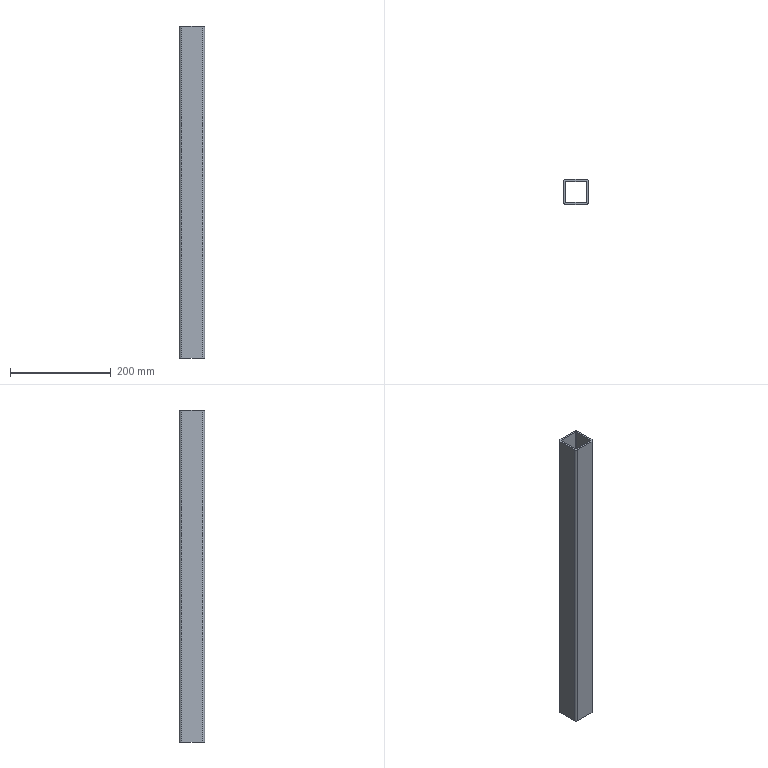Part | STEP file | 冲床-300配套压波_id966_x_t | 1 solid | 18 faces | box 50 x 50 x 660 mm | volume 472163 mm3 | plane 10 | cylinder 8 | commonest cylinder face diameters 2 x4 10 x4
STEP:
#1=CARTESIAN_POINT('',(1519.,-235.,-70.));
#2=VERTEX_POINT('',#1);
#3=CARTESIAN_POINT('',(1519.,-275.,-70.));
#4=VERTEX_POINT('',#3);
#5=CARTESIAN_POINT('',(1519.,-30.,-70.));
#6=DIRECTION('',(0.,-1.,0.));
#7=VECTOR('',#6,1.);
#8=LINE('',#5,#7);
#9=EDGE_CURVE('',#2,#4,#8,.T.);
#10=ORIENTED_EDGE('',*,*,#9,.F.);
#11=CARTESIAN_POINT('',(1520.,-234.,-70.));
#12=VERTEX_POINT('',#11);
#13=CARTESIAN_POINT('',(1520.,-235.,-70.));
#14=DIRECTION('',(0.,0.,1.));
#15=DIRECTION('',(1.,0.,0.));
#16=AXIS2_PLACEMENT_3D('',#13,#14,#15);
#17=CIRCLE('',#16,1.);
#18=EDGE_CURVE('',#12,#2,#17,.T.);
#19=ORIENTED_EDGE('',*,*,#18,.F.);
#20=CARTESIAN_POINT('',(1560.,-234.,-70.));
#21=VERTEX_POINT('',#20);
#22=CARTESIAN_POINT('',(365.,-234.,-70.));
#23=DIRECTION('',(-1.,0.,0.));
#24=VECTOR('',#23,1.);
#25=LINE('',#22,#24);
#26=EDGE_CURVE('',#21,#12,#25,.T.);
#27=ORIENTED_EDGE('',*,*,#26,.F.);
#28=CARTESIAN_POINT('',(1561.,-235.,-70.));
#29=VERTEX_POINT('',#28);
#30=CARTESIAN_POINT('',(1560.,-235.,-70.));
#31=DIRECTION('',(0.,0.,1.));
#32=DIRECTION('',(1.,0.,0.));
#33=AXIS2_PLACEMENT_3D('',#30,#31,#32);
#34=CIRCLE('',#33,1.);
#35=EDGE_CURVE('',#29,#21,#34,.T.);
#36=ORIENTED_EDGE('',*,*,#35,.F.);
#37=CARTESIAN_POINT('',(1561.,-275.,-70.));
#38=VERTEX_POINT('',#37);
#39=CARTESIAN_POINT('',(1561.,-30.,-70.));
#40=DIRECTION('',(0.,1.,0.));
#41=VECTOR('',#40,1.);
#42=LINE('',#39,#41);
#43=EDGE_CURVE('',#38,#29,#42,.T.);
#44=ORIENTED_EDGE('',*,*,#43,.F.);
#45=CARTESIAN_POINT('',(1560.,-276.,-70.));
#46=VERTEX_POINT('',#45);
#47=CARTESIAN_POINT('',(1560.,-275.,-70.));
#48=DIRECTION('',(0.,0.,1.));
#49=DIRECTION('',(1.,0.,0.));
#50=AXIS2_PLACEMENT_3D('',#47,#48,#49);
#51=CIRCLE('',#50,1.);
#52=EDGE_CURVE('',#46,#38,#51,.T.);
#53=ORIENTED_EDGE('',*,*,#52,.F.);
#54=CARTESIAN_POINT('',(1520.,-276.,-70.));
#55=VERTEX_POINT('',#54);
#56=CARTESIAN_POINT('',(365.,-276.,-70.));
#57=DIRECTION('',(1.,0.,0.));
#58=VECTOR('',#57,1.);
#59=LINE('',#56,#58);
#60=EDGE_CURVE('',#55,#46,#59,.T.);
#61=ORIENTED_EDGE('',*,*,#60,.F.);
#62=CARTESIAN_POINT('',(1520.,-275.,-70.));
#63=DIRECTION('',(0.,0.,1.));
#64=DIRECTION('',(1.,0.,0.));
#65=AXIS2_PLACEMENT_3D('',#62,#63,#64);
#66=CIRCLE('',#65,1.);
#67=EDGE_CURVE('',#4,#55,#66,.T.);
#68=ORIENTED_EDGE('',*,*,#67,.F.);
#69=EDGE_LOOP('',(#10,#19,#27,#36,#44,#53,#61,#68));
#70=FACE_BOUND('',#69,.T.);
#71=CARTESIAN_POINT('',(1515.,-235.,-70.));
#72=VERTEX_POINT('',#71);
#73=CARTESIAN_POINT('',(1515.,-275.,-70.));
#74=VERTEX_POINT('',#73);
#75=CARTESIAN_POINT('',(1515.,-30.,-70.));
#76=DIRECTION('',(0.,-1.,0.));
#77=VECTOR('',#76,1.);
#78=LINE('',#75,#77);
#79=EDGE_CURVE('',#72,#74,#78,.T.);
#80=ORIENTED_EDGE('',*,*,#79,.T.);
#81=CARTESIAN_POINT('',(1520.,-280.,-70.));
#82=VERTEX_POINT('',#81);
#83=CARTESIAN_POINT('',(1520.,-275.,-70.));
#84=DIRECTION('',(0.,0.,1.));
#85=DIRECTION('',(1.,0.,0.));
#86=AXIS2_PLACEMENT_3D('',#83,#84,#85);
#87=CIRCLE('',#86,5.);
#88=EDGE_CURVE('',#74,#82,#87,.T.);
#89=ORIENTED_EDGE('',*,*,#88,.T.);
#90=CARTESIAN_POINT('',(1560.,-280.,-70.));
#91=VERTEX_POINT('',#90);
#92=CARTESIAN_POINT('',(365.,-280.,-70.));
#93=DIRECTION('',(1.,0.,0.));
#94=VECTOR('',#93,1.);
#95=LINE('',#92,#94);
#96=EDGE_CURVE('',#82,#91,#95,.T.);
#97=ORIENTED_EDGE('',*,*,#96,.T.);
#98=CARTESIAN_POINT('',(1565.,-275.,-70.));
#99=VERTEX_POINT('',#98);
#100=CARTESIAN_POINT('',(1560.,-275.,-70.));
#101=DIRECTION('',(0.,0.,1.));
#102=DIRECTION('',(1.,0.,0.));
#103=AXIS2_PLACEMENT_3D('',#100,#101,#102);
#104=CIRCLE('',#103,5.);
#105=EDGE_CURVE('',#91,#99,#104,.T.);
#106=ORIENTED_EDGE('',*,*,#105,.T.);
#107=CARTESIAN_POINT('',(1565.,-235.,-70.));
#108=VERTEX_POINT('',#107);
#109=CARTESIAN_POINT('',(1565.,-30.,-70.));
#110=DIRECTION('',(0.,1.,0.));
#111=VECTOR('',#110,1.);
#112=LINE('',#109,#111);
#113=EDGE_CURVE('',#99,#108,#112,.T.);
#114=ORIENTED_EDGE('',*,*,#113,.T.);
#115=CARTESIAN_POINT('',(1560.,-230.,-70.));
#116=VERTEX_POINT('',#115);
#117=CARTESIAN_POINT('',(1560.,-235.,-70.));
#118=DIRECTION('',(0.,0.,1.));
#119=DIRECTION('',(1.,0.,0.));
#120=AXIS2_PLACEMENT_3D('',#117,#118,#119);
#121=CIRCLE('',#120,5.);
#122=EDGE_CURVE('',#108,#116,#121,.T.);
#123=ORIENTED_EDGE('',*,*,#122,.T.);
#124=CARTESIAN_POINT('',(1520.,-230.,-70.));
#125=VERTEX_POINT('',#124);
#126=CARTESIAN_POINT('',(365.,-230.,-70.));
#127=DIRECTION('',(-1.,0.,0.));
#128=VECTOR('',#127,1.);
#129=LINE('',#126,#128);
#130=EDGE_CURVE('',#116,#125,#129,.T.);
#131=ORIENTED_EDGE('',*,*,#130,.T.);
#132=CARTESIAN_POINT('',(1520.,-235.,-70.));
#133=DIRECTION('',(0.,0.,1.));
#134=DIRECTION('',(1.,0.,0.));
#135=AXIS2_PLACEMENT_3D('',#132,#133,#134);
#136=CIRCLE('',#135,5.);
#137=EDGE_CURVE('',#125,#72,#136,.T.);
#138=ORIENTED_EDGE('',*,*,#137,.T.);
#139=EDGE_LOOP('',(#80,#89,#97,#106,#114,#123,#131,#138));
#140=FACE_BOUND('',#139,.T.);
#141=CARTESIAN_POINT('',(365.,-30.,-70.));
#142=DIRECTION('',(0.,0.,1.));
#143=DIRECTION('',(1.,0.,0.));
#144=AXIS2_PLACEMENT_3D('',#141,#142,#143);
#145=PLANE('',#144);
#146=ADVANCED_FACE('',(#70,#140),#145,.T.);
#147=CARTESIAN_POINT('',(1520.,-230.,-730.));
#148=VERTEX_POINT('',#147);
#149=CARTESIAN_POINT('',(1520.,-230.,-740.));
#150=DIRECTION('',(0.,0.,-1.));
#151=VECTOR('',#150,1.);
#152=LINE('',#149,#151);
#153=EDGE_CURVE('',#125,#148,#152,.T.);
#154=ORIENTED_EDGE('',*,*,#153,.T.);
#155=CARTESIAN_POINT('',(1515.,-235.,-730.));
#156=VERTEX_POINT('',#155);
#157=CARTESIAN_POINT('',(1520.,-235.,-730.));
#158=DIRECTION('',(0.,0.,1.));
#159=DIRECTION('',(1.,0.,0.));
#160=AXIS2_PLACEMENT_3D('',#157,#158,#159);
#161=CIRCLE('',#160,5.);
#162=EDGE_CURVE('',#148,#156,#161,.T.);
#163=ORIENTED_EDGE('',*,*,#162,.T.);
#164=CARTESIAN_POINT('',(1515.,-235.,-740.));
#165=DIRECTION('',(0.,0.,-1.));
#166=VECTOR('',#165,1.);
#167=LINE('',#164,#166);
#168=EDGE_CURVE('',#72,#156,#167,.T.);
#169=ORIENTED_EDGE('',*,*,#168,.F.);
#170=ORIENTED_EDGE('',*,*,#137,.F.);
#171=EDGE_LOOP('',(#154,#163,#169,#170));
#172=FACE_OUTER_BOUND('',#171,.T.);
#173=CARTESIAN_POINT('',(1520.,-235.,-740.));
#174=DIRECTION('',(0.,0.,1.));
#175=DIRECTION('',(1.,0.,0.));
#176=AXIS2_PLACEMENT_3D('',#173,#174,#175);
#177=CYLINDRICAL_SURFACE('',#176,5.);
#178=ADVANCED_FACE('',(#172),#177,.T.);
#179=CARTESIAN_POINT('',(1560.,-230.,-730.));
#180=VERTEX_POINT('',#179);
#181=CARTESIAN_POINT('',(1560.,-230.,-740.));
#182=DIRECTION('',(0.,0.,-1.));
#183=VECTOR('',#182,1.);
#184=LINE('',#181,#183);
#185=EDGE_CURVE('',#116,#180,#184,.T.);
#186=ORIENTED_EDGE('',*,*,#185,.T.);
#187=CARTESIAN_POINT('',(1520.,-230.,-730.));
#188=DIRECTION('',(-1.,0.,0.));
#189=VECTOR('',#188,1.);
#190=LINE('',#187,#189);
#191=EDGE_CURVE('',#180,#148,#190,.T.);
#192=ORIENTED_EDGE('',*,*,#191,.T.);
#193=ORIENTED_EDGE('',*,*,#153,.F.);
#194=ORIENTED_EDGE('',*,*,#130,.F.);
#195=EDGE_LOOP('',(#186,#192,#193,#194));
#196=FACE_OUTER_BOUND('',#195,.T.);
#197=CARTESIAN_POINT('',(1520.,-230.,-740.));
#198=DIRECTION('',(0.,1.,0.));
#199=DIRECTION('',(1.,0.,0.));
#200=AXIS2_PLACEMENT_3D('',#197,#198,#199);
#201=PLANE('',#200);
#202=ADVANCED_FACE('',(#196),#201,.T.);
#203=CARTESIAN_POINT('',(1565.,-235.,-730.));
#204=VERTEX_POINT('',#203);
#205=CARTESIAN_POINT('',(1565.,-235.,-740.));
#206=DIRECTION('',(0.,0.,-1.));
#207=VECTOR('',#206,1.);
#208=LINE('',#205,#207);
#209=EDGE_CURVE('',#108,#204,#208,.T.);
#210=ORIENTED_EDGE('',*,*,#209,.T.);
#211=CARTESIAN_POINT('',(1560.,-235.,-730.));
#212=DIRECTION('',(0.,0.,1.));
#213=DIRECTION('',(1.,0.,0.));
#214=AXIS2_PLACEMENT_3D('',#211,#212,#213);
#215=CIRCLE('',#214,5.);
#216=EDGE_CURVE('',#204,#180,#215,.T.);
#217=ORIENTED_EDGE('',*,*,#216,.T.);
#218=ORIENTED_EDGE('',*,*,#185,.F.);
#219=ORIENTED_EDGE('',*,*,#122,.F.);
#220=EDGE_LOOP('',(#210,#217,#218,#219));
#221=FACE_OUTER_BOUND('',#220,.T.);
#222=CARTESIAN_POINT('',(1560.,-235.,-740.));
#223=DIRECTION('',(0.,0.,1.));
#224=DIRECTION('',(1.,0.,0.));
#225=AXIS2_PLACEMENT_3D('',#222,#223,#224);
#226=CYLINDRICAL_SURFACE('',#225,5.);
#227=ADVANCED_FACE('',(#221),#226,.T.);
#228=CARTESIAN_POINT('',(1565.,-275.,-730.));
#229=VERTEX_POINT('',#228);
#230=CARTESIAN_POINT('',(1565.,-275.,-740.));
#231=DIRECTION('',(0.,0.,-1.));
#232=VECTOR('',#231,1.);
#233=LINE('',#230,#232);
#234=EDGE_CURVE('',#99,#229,#233,.T.);
#235=ORIENTED_EDGE('',*,*,#234,.T.);
#236=CARTESIAN_POINT('',(1565.,-235.,-730.));
#237=DIRECTION('',(0.,1.,0.));
#238=VECTOR('',#237,1.);
#239=LINE('',#236,#238);
#240=EDGE_CURVE('',#229,#204,#239,.T.);
#241=ORIENTED_EDGE('',*,*,#240,.T.);
#242=ORIENTED_EDGE('',*,*,#209,.F.);
#243=ORIENTED_EDGE('',*,*,#113,.F.);
#244=EDGE_LOOP('',(#235,#241,#242,#243));
#245=FACE_OUTER_BOUND('',#244,.T.);
#246=CARTESIAN_POINT('',(1565.,-235.,-740.));
#247=DIRECTION('',(1.,0.,0.));
#248=DIRECTION('',(0.,0.,-1.));
#249=AXIS2_PLACEMENT_3D('',#246,#247,#248);
#250=PLANE('',#249);
#251=ADVANCED_FACE('',(#245),#250,.T.);
#252=CARTESIAN_POINT('',(1560.,-280.,-730.));
#253=VERTEX_POINT('',#252);
#254=CARTESIAN_POINT('',(1560.,-280.,-740.));
#255=DIRECTION('',(0.,0.,-1.));
#256=VECTOR('',#255,1.);
#257=LINE('',#254,#256);
#258=EDGE_CURVE('',#91,#253,#257,.T.);
#259=ORIENTED_EDGE('',*,*,#258,.T.);
#260=CARTESIAN_POINT('',(1560.,-275.,-730.));
#261=DIRECTION('',(0.,0.,1.));
#262=DIRECTION('',(1.,0.,0.));
#263=AXIS2_PLACEMENT_3D('',#260,#261,#262);
#264=CIRCLE('',#263,5.);
#265=EDGE_CURVE('',#253,#229,#264,.T.);
#266=ORIENTED_EDGE('',*,*,#265,.T.);
#267=ORIENTED_EDGE('',*,*,#234,.F.);
#268=ORIENTED_EDGE('',*,*,#105,.F.);
#269=EDGE_LOOP('',(#259,#266,#267,#268));
#270=FACE_OUTER_BOUND('',#269,.T.);
#271=CARTESIAN_POINT('',(1560.,-275.,-740.));
#272=DIRECTION('',(0.,0.,1.));
#273=DIRECTION('',(1.,0.,0.));
#274=AXIS2_PLACEMENT_3D('',#271,#272,#273);
#275=CYLINDRICAL_SURFACE('',#274,5.);
#276=ADVANCED_FACE('',(#270),#275,.T.);
#277=CARTESIAN_POINT('',(1519.,-275.,-730.));
#278=VERTEX_POINT('',#277);
#279=CARTESIAN_POINT('',(1520.,-276.,-730.));
#280=VERTEX_POINT('',#279);
#281=CARTESIAN_POINT('',(1520.,-275.,-730.));
#282=DIRECTION('',(0.,0.,1.));
#283=DIRECTION('',(1.,0.,0.));
#284=AXIS2_PLACEMENT_3D('',#281,#282,#283);
#285=CIRCLE('',#284,1.);
#286=EDGE_CURVE('',#278,#280,#285,.T.);
#287=ORIENTED_EDGE('',*,*,#286,.T.);
#288=CARTESIAN_POINT('',(1560.,-276.,-730.));
#289=VERTEX_POINT('',#288);
#290=CARTESIAN_POINT('',(1520.,-276.,-730.));
#291=DIRECTION('',(1.,0.,0.));
#292=VECTOR('',#291,1.);
#293=LINE('',#290,#292);
#294=EDGE_CURVE('',#280,#289,#293,.T.);
#295=ORIENTED_EDGE('',*,*,#294,.T.);
#296=CARTESIAN_POINT('',(1561.,-275.,-730.));
#297=VERTEX_POINT('',#296);
#298=CARTESIAN_POINT('',(1560.,-275.,-730.));
#299=DIRECTION('',(0.,0.,1.));
#300=DIRECTION('',(1.,0.,0.));
#301=AXIS2_PLACEMENT_3D('',#298,#299,#300);
#302=CIRCLE('',#301,1.);
#303=EDGE_CURVE('',#289,#297,#302,.T.);
#304=ORIENTED_EDGE('',*,*,#303,.T.);
#305=CARTESIAN_POINT('',(1561.,-235.,-730.));
#306=VERTEX_POINT('',#305);
#307=CARTESIAN_POINT('',(1561.,-235.,-730.));
#308=DIRECTION('',(0.,1.,0.));
#309=VECTOR('',#308,1.);
#310=LINE('',#307,#309);
#311=EDGE_CURVE('',#297,#306,#310,.T.);
#312=ORIENTED_EDGE('',*,*,#311,.T.);
#313=CARTESIAN_POINT('',(1560.,-234.,-730.));
#314=VERTEX_POINT('',#313);
#315=CARTESIAN_POINT('',(1560.,-235.,-730.));
#316=DIRECTION('',(0.,0.,1.));
#317=DIRECTION('',(1.,0.,0.));
#318=AXIS2_PLACEMENT_3D('',#315,#316,#317);
#319=CIRCLE('',#318,1.);
#320=EDGE_CURVE('',#306,#314,#319,.T.);
#321=ORIENTED_EDGE('',*,*,#320,.T.);
#322=CARTESIAN_POINT('',(1520.,-234.,-730.));
#323=VERTEX_POINT('',#322);
#324=CARTESIAN_POINT('',(1520.,-234.,-730.));
#325=DIRECTION('',(-1.,0.,0.));
#326=VECTOR('',#325,1.);
#327=LINE('',#324,#326);
#328=EDGE_CURVE('',#314,#323,#327,.T.);
#329=ORIENTED_EDGE('',*,*,#328,.T.);
#330=CARTESIAN_POINT('',(1519.,-235.,-730.));
#331=VERTEX_POINT('',#330);
#332=CARTESIAN_POINT('',(1520.,-235.,-730.));
#333=DIRECTION('',(0.,0.,1.));
#334=DIRECTION('',(1.,0.,0.));
#335=AXIS2_PLACEMENT_3D('',#332,#333,#334);
#336=CIRCLE('',#335,1.);
#337=EDGE_CURVE('',#323,#331,#336,.T.);
#338=ORIENTED_EDGE('',*,*,#337,.T.);
#339=CARTESIAN_POINT('',(1519.,-235.,-730.));
#340=DIRECTION('',(0.,-1.,0.));
#341=VECTOR('',#340,1.);
#342=LINE('',#339,#341);
#343=EDGE_CURVE('',#331,#278,#342,.T.);
#344=ORIENTED_EDGE('',*,*,#343,.T.);
#345=EDGE_LOOP('',(#287,#295,#304,#312,#321,#329,#338,#344));
#346=FACE_BOUND('',#345,.T.);
#347=CARTESIAN_POINT('',(1515.,-275.,-730.));
#348=VERTEX_POINT('',#347);
#349=CARTESIAN_POINT('',(1515.,-235.,-730.));
#350=DIRECTION('',(0.,-1.,0.));
#351=VECTOR('',#350,1.);
#352=LINE('',#349,#351);
#353=EDGE_CURVE('',#156,#348,#352,.T.);
#354=ORIENTED_EDGE('',*,*,#353,.F.);
#355=ORIENTED_EDGE('',*,*,#162,.F.);
#356=ORIENTED_EDGE('',*,*,#191,.F.);
#357=ORIENTED_EDGE('',*,*,#216,.F.);
#358=ORIENTED_EDGE('',*,*,#240,.F.);
#359=ORIENTED_EDGE('',*,*,#265,.F.);
#360=CARTESIAN_POINT('',(1520.,-280.,-730.));
#361=VERTEX_POINT('',#360);
#362=CARTESIAN_POINT('',(1520.,-280.,-730.));
#363=DIRECTION('',(1.,0.,0.));
#364=VECTOR('',#363,1.);
#365=LINE('',#362,#364);
#366=EDGE_CURVE('',#361,#253,#365,.T.);
#367=ORIENTED_EDGE('',*,*,#366,.F.);
#368=CARTESIAN_POINT('',(1520.,-275.,-730.));
#369=DIRECTION('',(0.,0.,1.));
#370=DIRECTION('',(1.,0.,0.));
#371=AXIS2_PLACEMENT_3D('',#368,#369,#370);
#372=CIRCLE('',#371,5.);
#373=EDGE_CURVE('',#348,#361,#372,.T.);
#374=ORIENTED_EDGE('',*,*,#373,.F.);
#375=EDGE_LOOP('',(#354,#355,#356,#357,#358,#359,#367,#374));
#376=FACE_BOUND('',#375,.T.);
#377=CARTESIAN_POINT('',(1520.,-235.,-730.));
#378=DIRECTION('',(0.,0.,1.));
#379=DIRECTION('',(1.,0.,0.));
#380=AXIS2_PLACEMENT_3D('',#377,#378,#379);
#381=PLANE('',#380);
#382=ADVANCED_FACE('',(#346,#376),#381,.F.);
#383=CARTESIAN_POINT('',(1520.,-280.,-740.));
#384=DIRECTION('',(0.,0.,-1.));
#385=VECTOR('',#384,1.);
#386=LINE('',#383,#385);
#387=EDGE_CURVE('',#82,#361,#386,.T.);
#388=ORIENTED_EDGE('',*,*,#387,.T.);
#389=ORIENTED_EDGE('',*,*,#366,.T.);
#390=ORIENTED_EDGE('',*,*,#258,.F.);
#391=ORIENTED_EDGE('',*,*,#96,.F.);
#392=EDGE_LOOP('',(#388,#389,#390,#391));
#393=FACE_OUTER_BOUND('',#392,.T.);
#394=CARTESIAN_POINT('',(1560.,-280.,-740.));
#395=DIRECTION('',(0.,-1.,0.));
#396=DIRECTION('',(-1.,0.,0.));
#397=AXIS2_PLACEMENT_3D('',#394,#395,#396);
#398=PLANE('',#397);
#399=ADVANCED_FACE('',(#393),#398,.T.);
#400=ORIENTED_EDGE('',*,*,#168,.T.);
#401=ORIENTED_EDGE('',*,*,#353,.T.);
#402=CARTESIAN_POINT('',(1515.,-275.,-740.));
#403=DIRECTION('',(0.,0.,-1.));
#404=VECTOR('',#403,1.);
#405=LINE('',#402,#404);
#406=EDGE_CURVE('',#74,#348,#405,.T.);
#407=ORIENTED_EDGE('',*,*,#406,.F.);
#408=ORIENTED_EDGE('',*,*,#79,.F.);
#409=EDGE_LOOP('',(#400,#401,#407,#408));
#410=FACE_OUTER_BOUND('',#409,.T.);
#411=CARTESIAN_POINT('',(1515.,-275.,-740.));
#412=DIRECTION('',(-1.,0.,0.));
#413=DIRECTION('',(0.,0.,1.));
#414=AXIS2_PLACEMENT_3D('',#411,#412,#413);
#415=PLANE('',#414);
#416=ADVANCED_FACE('',(#410),#415,.T.);
#417=ORIENTED_EDGE('',*,*,#406,.T.);
#418=ORIENTED_EDGE('',*,*,#373,.T.);
#419=ORIENTED_EDGE('',*,*,#387,.F.);
#420=ORIENTED_EDGE('',*,*,#88,.F.);
#421=EDGE_LOOP('',(#417,#418,#419,#420));
#422=FACE_OUTER_BOUND('',#421,.T.);
#423=CARTESIAN_POINT('',(1520.,-275.,-740.));
#424=DIRECTION('',(0.,0.,1.));
#425=DIRECTION('',(1.,0.,0.));
#426=AXIS2_PLACEMENT_3D('',#423,#424,#425);
#427=CYLINDRICAL_SURFACE('',#426,5.);
#428=ADVANCED_FACE('',(#422),#427,.T.);
#429=CARTESIAN_POINT('',(1520.,-234.,-740.));
#430=DIRECTION('',(0.,0.,-1.));
#431=VECTOR('',#430,1.);
#432=LINE('',#429,#431);
#433=EDGE_CURVE('',#12,#323,#432,.T.);
#434=ORIENTED_EDGE('',*,*,#433,.F.);
#435=ORIENTED_EDGE('',*,*,#18,.T.);
#436=CARTESIAN_POINT('',(1519.,-235.,-740.));
#437=DIRECTION('',(0.,0.,-1.));
#438=VECTOR('',#437,1.);
#439=LINE('',#436,#438);
#440=EDGE_CURVE('',#2,#331,#439,.T.);
#441=ORIENTED_EDGE('',*,*,#440,.T.);
#442=ORIENTED_EDGE('',*,*,#337,.F.);
#443=EDGE_LOOP('',(#434,#435,#441,#442));
#444=FACE_OUTER_BOUND('',#443,.T.);
#445=CARTESIAN_POINT('',(1520.,-235.,-740.));
#446=DIRECTION('',(0.,0.,1.));
#447=DIRECTION('',(1.,0.,0.));
#448=AXIS2_PLACEMENT_3D('',#445,#446,#447);
#449=CYLINDRICAL_SURFACE('',#448,1.);
#450=ADVANCED_FACE('',(#444),#449,.F.);
#451=CARTESIAN_POINT('',(1560.,-234.,-740.));
#452=DIRECTION('',(0.,0.,-1.));
#453=VECTOR('',#452,1.);
#454=LINE('',#451,#453);
#455=EDGE_CURVE('',#21,#314,#454,.T.);
#456=ORIENTED_EDGE('',*,*,#455,.F.);
#457=ORIENTED_EDGE('',*,*,#26,.T.);
#458=ORIENTED_EDGE('',*,*,#433,.T.);
#459=ORIENTED_EDGE('',*,*,#328,.F.);
#460=EDGE_LOOP('',(#456,#457,#458,#459));
#461=FACE_OUTER_BOUND('',#460,.T.);
#462=CARTESIAN_POINT('',(1520.,-234.,-740.));
#463=DIRECTION('',(0.,1.,0.));
#464=DIRECTION('',(1.,0.,0.));
#465=AXIS2_PLACEMENT_3D('',#462,#463,#464);
#466=PLANE('',#465);
#467=ADVANCED_FACE('',(#461),#466,.F.);
#468=CARTESIAN_POINT('',(1561.,-235.,-740.));
#469=DIRECTION('',(0.,0.,-1.));
#470=VECTOR('',#469,1.);
#471=LINE('',#468,#470);
#472=EDGE_CURVE('',#29,#306,#471,.T.);
#473=ORIENTED_EDGE('',*,*,#472,.F.);
#474=ORIENTED_EDGE('',*,*,#35,.T.);
#475=ORIENTED_EDGE('',*,*,#455,.T.);
#476=ORIENTED_EDGE('',*,*,#320,.F.);
#477=EDGE_LOOP('',(#473,#474,#475,#476));
#478=FACE_OUTER_BOUND('',#477,.T.);
#479=CARTESIAN_POINT('',(1560.,-235.,-740.));
#480=DIRECTION('',(0.,0.,1.));
#481=DIRECTION('',(1.,0.,0.));
#482=AXIS2_PLACEMENT_3D('',#479,#480,#481);
#483=CYLINDRICAL_SURFACE('',#482,1.);
#484=ADVANCED_FACE('',(#478),#483,.F.);
#485=CARTESIAN_POINT('',(1561.,-275.,-740.));
#486=DIRECTION('',(0.,0.,-1.));
#487=VECTOR('',#486,1.);
#488=LINE('',#485,#487);
#489=EDGE_CURVE('',#38,#297,#488,.T.);
#490=ORIENTED_EDGE('',*,*,#489,.F.);
#491=ORIENTED_EDGE('',*,*,#43,.T.);
#492=ORIENTED_EDGE('',*,*,#472,.T.);
#493=ORIENTED_EDGE('',*,*,#311,.F.);
#494=EDGE_LOOP('',(#490,#491,#492,#493));
#495=FACE_OUTER_BOUND('',#494,.T.);
#496=CARTESIAN_POINT('',(1561.,-235.,-740.));
#497=DIRECTION('',(1.,0.,0.));
#498=DIRECTION('',(0.,0.,-1.));
#499=AXIS2_PLACEMENT_3D('',#496,#497,#498);
#500=PLANE('',#499);
#501=ADVANCED_FACE('',(#495),#500,.F.);
#502=CARTESIAN_POINT('',(1560.,-276.,-740.));
#503=DIRECTION('',(0.,0.,-1.));
#504=VECTOR('',#503,1.);
#505=LINE('',#502,#504);
#506=EDGE_CURVE('',#46,#289,#505,.T.);
#507=ORIENTED_EDGE('',*,*,#506,.F.);
#508=ORIENTED_EDGE('',*,*,#52,.T.);
#509=ORIENTED_EDGE('',*,*,#489,.T.);
#510=ORIENTED_EDGE('',*,*,#303,.F.);
#511=EDGE_LOOP('',(#507,#508,#509,#510));
#512=FACE_OUTER_BOUND('',#511,.T.);
#513=CARTESIAN_POINT('',(1560.,-275.,-740.));
#514=DIRECTION('',(0.,0.,1.));
#515=DIRECTION('',(1.,0.,0.));
#516=AXIS2_PLACEMENT_3D('',#513,#514,#515);
#517=CYLINDRICAL_SURFACE('',#516,1.);
#518=ADVANCED_FACE('',(#512),#517,.F.);
#519=CARTESIAN_POINT('',(1520.,-276.,-740.));
#520=DIRECTION('',(0.,0.,-1.));
#521=VECTOR('',#520,1.);
#522=LINE('',#519,#521);
#523=EDGE_CURVE('',#55,#280,#522,.T.);
#524=ORIENTED_EDGE('',*,*,#523,.F.);
#525=ORIENTED_EDGE('',*,*,#60,.T.);
#526=ORIENTED_EDGE('',*,*,#506,.T.);
#527=ORIENTED_EDGE('',*,*,#294,.F.);
#528=EDGE_LOOP('',(#524,#525,#526,#527));
#529=FACE_OUTER_BOUND('',#528,.T.);
#530=CARTESIAN_POINT('',(1560.,-276.,-740.));
#531=DIRECTION('',(0.,-1.,0.));
#532=DIRECTION('',(-1.,0.,0.));
#533=AXIS2_PLACEMENT_3D('',#530,#531,#532);
#534=PLANE('',#533);
#535=ADVANCED_FACE('',(#529),#534,.F.);
#536=ORIENTED_EDGE('',*,*,#440,.F.);
#537=ORIENTED_EDGE('',*,*,#9,.T.);
#538=CARTESIAN_POINT('',(1519.,-275.,-740.));
#539=DIRECTION('',(0.,0.,-1.));
#540=VECTOR('',#539,1.);
#541=LINE('',#538,#540);
#542=EDGE_CURVE('',#4,#278,#541,.T.);
#543=ORIENTED_EDGE('',*,*,#542,.T.);
#544=ORIENTED_EDGE('',*,*,#343,.F.);
#545=EDGE_LOOP('',(#536,#537,#543,#544));
#546=FACE_OUTER_BOUND('',#545,.T.);
#547=CARTESIAN_POINT('',(1519.,-275.,-740.));
#548=DIRECTION('',(-1.,0.,0.));
#549=DIRECTION('',(0.,0.,1.));
#550=AXIS2_PLACEMENT_3D('',#547,#548,#549);
#551=PLANE('',#550);
#552=ADVANCED_FACE('',(#546),#551,.F.);
#553=ORIENTED_EDGE('',*,*,#542,.F.);
#554=ORIENTED_EDGE('',*,*,#67,.T.);
#555=ORIENTED_EDGE('',*,*,#523,.T.);
#556=ORIENTED_EDGE('',*,*,#286,.F.);
#557=EDGE_LOOP('',(#553,#554,#555,#556));
#558=FACE_OUTER_BOUND('',#557,.T.);
#559=CARTESIAN_POINT('',(1520.,-275.,-740.));
#560=DIRECTION('',(0.,0.,1.));
#561=DIRECTION('',(1.,0.,0.));
#562=AXIS2_PLACEMENT_3D('',#559,#560,#561);
#563=CYLINDRICAL_SURFACE('',#562,1.);
#564=ADVANCED_FACE('',(#558),#563,.F.);
#565=CLOSED_SHELL('',(#146,#178,#202,#227,#251,#276,#382,#399,#416,#428,#450,#467,#484,#501,#518,#535,#552,#564));
#566=MANIFOLD_SOLID_BREP('',#565);
#567=(LENGTH_UNIT()NAMED_UNIT(*)SI_UNIT(.MILLI.,.METRE.));
#568=UNCERTAINTY_MEASURE_WITH_UNIT(LENGTH_MEASURE(0.00002),#567,'','');
#569=(NAMED_UNIT(*)PLANE_ANGLE_UNIT()SI_UNIT($,.RADIAN.));
#570=PLANE_ANGLE_MEASURE_WITH_UNIT(PLANE_ANGLE_MEASURE(0.01745),#569);
#571=DIMENSIONAL_EXPONENTS(0.,0.,0.,0.,0.,0.,0.);
#572=(CONVERSION_BASED_UNIT('DEGREE',#570)NAMED_UNIT(#571)PLANE_ANGLE_UNIT());
#573=(NAMED_UNIT(*)SI_UNIT($,.STERADIAN.)SOLID_ANGLE_UNIT());
#574=(GEOMETRIC_REPRESENTATION_CONTEXT(3)GLOBAL_UNCERTAINTY_ASSIGNED_CONTEXT((#568))GLOBAL_UNIT_ASSIGNED_CONTEXT((#567,#572,#573))REPRESENTATION_CONTEXT('',''));
#575=ADVANCED_BREP_SHAPE_REPRESENTATION('',(#566),#574);